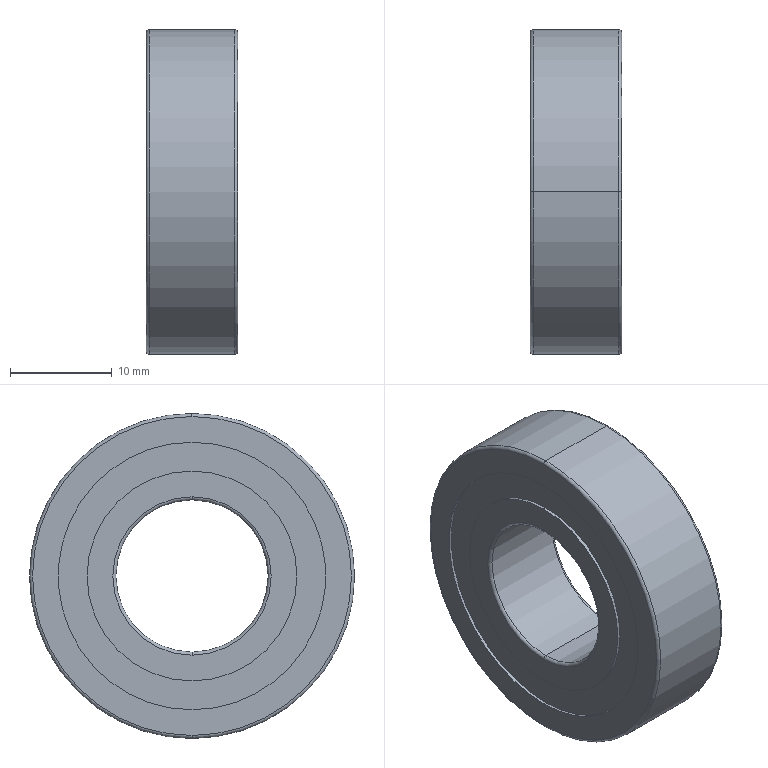Part | STEP file | 6002ZZ_Rolling bearings 6002 GB 276-94 | 1 solid | 116 faces | box 9 x 32 x 32 mm | volume 4596 mm3 | torus 56 | sphere 32 | cylinder 20 | plane 8 | commonest cylinder face diameters 20.667 x8 26.333 x8 15 x2 32 x2